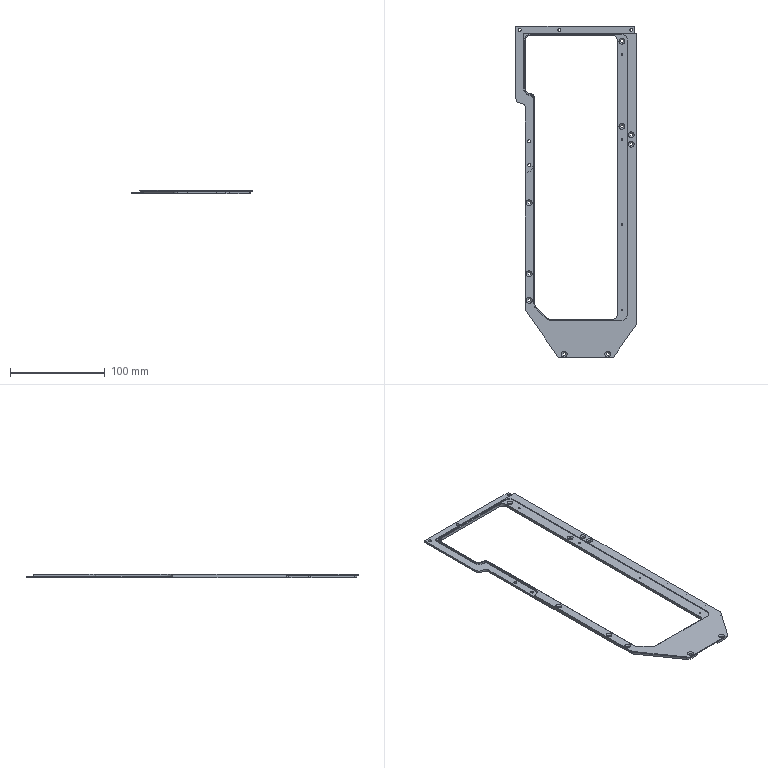Part | 1 solid | 123 faces | box 127 x 351 x 4 mm | volume 39794 mm3 | cylinder 66 | plane 39 | cone 18 | commonest cylinder face diameters 3.2 x26 10 x16 1.6 x8 12 x6 4 x4 3 x2